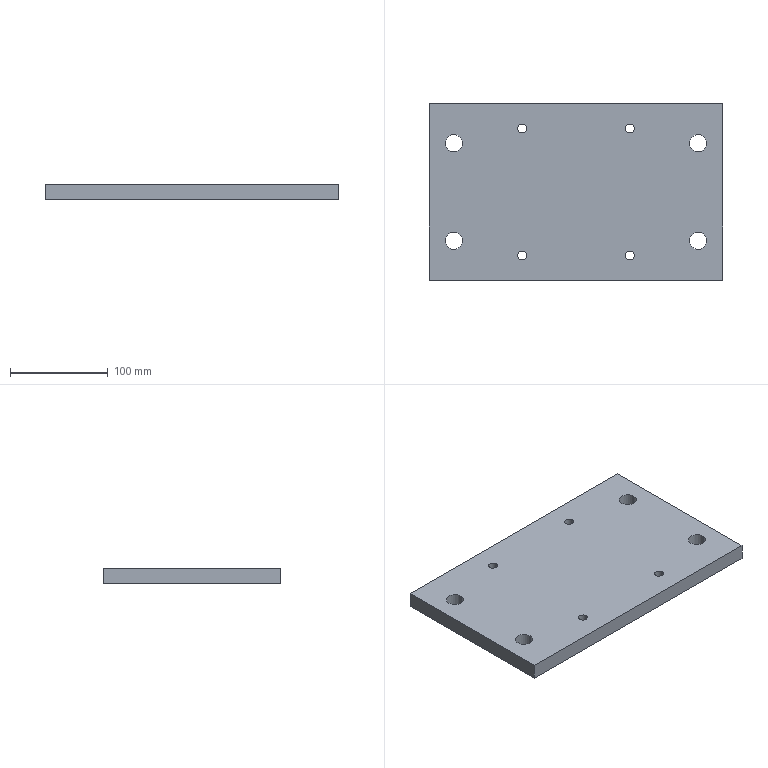Part | STEP file | 1 solid | 22 faces | box 300 x 180 x 16 mm | volume 844535 mm3 | cylinder 16 | plane 6 | commonest cylinder face diameters 9 x8 17.5 x8